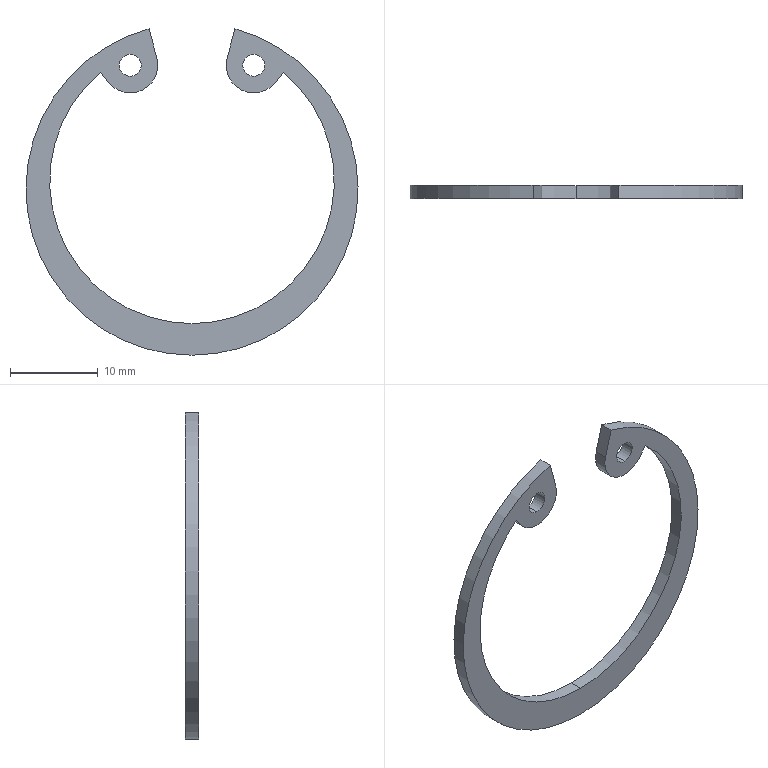Part | SolidWorks | features Extrusion 1 | 1 solid | 18 faces | box 37.8 x 1.5 x 37.156 mm | volume 475.123 mm3 | cylinder 12 | plane 6 | commonest cylinder face diameters 2.5 x4 6.28 x4 32.4 x2 37.8 x2
STEP:
#1=CARTESIAN_POINT('',(7.03,1.5,12.855));
#2=VERTEX_POINT('',#1);
#3=CARTESIAN_POINT('',(7.03,1.5,15.355));
#4=VERTEX_POINT('',#3);
#5=CARTESIAN_POINT('',(7.03,1.5,14.105));
#6=DIRECTION('',(0.,1.,0.));
#7=DIRECTION('',(0.,0.,-1.));
#8=AXIS2_PLACEMENT_3D('',#5,#6,#7);
#9=CIRCLE('',#8,1.25);
#10=EDGE_CURVE('',#2,#4,#9,.T.);
#11=ORIENTED_EDGE('',*,*,#10,.T.);
#12=CARTESIAN_POINT('',(7.03,0.,15.355));
#13=VERTEX_POINT('',#12);
#14=CARTESIAN_POINT('',(7.03,1.5,15.355));
#15=DIRECTION('',(0.,-1.,0.));
#16=VECTOR('',#15,1000.);
#17=LINE('',#14,#16);
#18=EDGE_CURVE('',#4,#13,#17,.T.);
#19=ORIENTED_EDGE('',*,*,#18,.T.);
#20=CARTESIAN_POINT('',(7.03,0.,12.855));
#21=VERTEX_POINT('',#20);
#22=CARTESIAN_POINT('',(7.03,0.,14.105));
#23=DIRECTION('',(0.,1.,0.));
#24=DIRECTION('',(0.,0.,-1.));
#25=AXIS2_PLACEMENT_3D('',#22,#23,#24);
#26=CIRCLE('',#25,1.25);
#27=EDGE_CURVE('',#21,#13,#26,.T.);
#28=ORIENTED_EDGE('',*,*,#27,.F.);
#29=CARTESIAN_POINT('',(7.03,1.5,12.855));
#30=DIRECTION('',(0.,-1.,0.));
#31=VECTOR('',#30,1000.);
#32=LINE('',#29,#31);
#33=EDGE_CURVE('',#2,#21,#32,.T.);
#34=ORIENTED_EDGE('',*,*,#33,.F.);
#35=EDGE_LOOP('',(#11,#19,#28,#34));
#36=FACE_OUTER_BOUND('',#35,.T.);
#37=CARTESIAN_POINT('',(7.03,1.5,14.105));
#38=DIRECTION('',(0.,-1.,0.));
#39=DIRECTION('',(0.,0.,-1.));
#40=AXIS2_PLACEMENT_3D('',#37,#38,#39);
#41=CYLINDRICAL_SURFACE('',#40,1.25);
#42=ADVANCED_FACE('',(#36),#41,.F.);
#43=CARTESIAN_POINT('',(-7.03,1.5,12.855));
#44=VERTEX_POINT('',#43);
#45=CARTESIAN_POINT('',(-7.03,1.5,15.355));
#46=VERTEX_POINT('',#45);
#47=CARTESIAN_POINT('',(-7.03,1.5,14.105));
#48=DIRECTION('',(0.,1.,0.));
#49=DIRECTION('',(0.,0.,1.));
#50=AXIS2_PLACEMENT_3D('',#47,#48,#49);
#51=CIRCLE('',#50,1.25);
#52=EDGE_CURVE('',#44,#46,#51,.T.);
#53=ORIENTED_EDGE('',*,*,#52,.T.);
#54=CARTESIAN_POINT('',(-7.03,0.,15.355));
#55=VERTEX_POINT('',#54);
#56=CARTESIAN_POINT('',(-7.03,1.5,15.355));
#57=DIRECTION('',(0.,-1.,0.));
#58=VECTOR('',#57,1000.);
#59=LINE('',#56,#58);
#60=EDGE_CURVE('',#46,#55,#59,.T.);
#61=ORIENTED_EDGE('',*,*,#60,.T.);
#62=CARTESIAN_POINT('',(-7.03,0.,12.855));
#63=VERTEX_POINT('',#62);
#64=CARTESIAN_POINT('',(-7.03,0.,14.105));
#65=DIRECTION('',(0.,1.,0.));
#66=DIRECTION('',(0.,0.,1.));
#67=AXIS2_PLACEMENT_3D('',#64,#65,#66);
#68=CIRCLE('',#67,1.25);
#69=EDGE_CURVE('',#63,#55,#68,.T.);
#70=ORIENTED_EDGE('',*,*,#69,.F.);
#71=CARTESIAN_POINT('',(-7.03,1.5,12.855));
#72=DIRECTION('',(0.,-1.,0.));
#73=VECTOR('',#72,1000.);
#74=LINE('',#71,#73);
#75=EDGE_CURVE('',#44,#63,#74,.T.);
#76=ORIENTED_EDGE('',*,*,#75,.F.);
#77=EDGE_LOOP('',(#53,#61,#70,#76));
#78=FACE_OUTER_BOUND('',#77,.T.);
#79=CARTESIAN_POINT('',(-7.03,1.5,14.105));
#80=DIRECTION('',(0.,-1.,0.));
#81=DIRECTION('',(0.,0.,-1.));
#82=AXIS2_PLACEMENT_3D('',#79,#80,#81);
#83=CYLINDRICAL_SURFACE('',#82,1.25);
#84=ADVANCED_FACE('',(#78),#83,.F.);
#85=CARTESIAN_POINT('',(0.,1.5,-18.9));
#86=VERTEX_POINT('',#85);
#87=CARTESIAN_POINT('',(-4.892,1.5,18.256));
#88=VERTEX_POINT('',#87);
#89=CARTESIAN_POINT('',(0.,1.5,0.));
#90=DIRECTION('',(0.,1.,0.));
#91=DIRECTION('',(0.,0.,1.));
#92=AXIS2_PLACEMENT_3D('',#89,#90,#91);
#93=CIRCLE('',#92,18.9);
#94=EDGE_CURVE('',#86,#88,#93,.T.);
#95=ORIENTED_EDGE('',*,*,#94,.F.);
#96=CARTESIAN_POINT('',(0.,0.,-18.9));
#97=VERTEX_POINT('',#96);
#98=CARTESIAN_POINT('',(0.,1.5,-18.9));
#99=DIRECTION('',(0.,-1.,0.));
#100=VECTOR('',#99,1000.);
#101=LINE('',#98,#100);
#102=EDGE_CURVE('',#86,#97,#101,.T.);
#103=ORIENTED_EDGE('',*,*,#102,.T.);
#104=CARTESIAN_POINT('',(-4.892,0.,18.256));
#105=VERTEX_POINT('',#104);
#106=CARTESIAN_POINT('',(0.,0.,0.));
#107=DIRECTION('',(0.,1.,0.));
#108=DIRECTION('',(0.,0.,1.));
#109=AXIS2_PLACEMENT_3D('',#106,#107,#108);
#110=CIRCLE('',#109,18.9);
#111=EDGE_CURVE('',#97,#105,#110,.T.);
#112=ORIENTED_EDGE('',*,*,#111,.T.);
#113=CARTESIAN_POINT('',(-4.892,1.5,18.256));
#114=DIRECTION('',(0.,-1.,0.));
#115=VECTOR('',#114,1000.);
#116=LINE('',#113,#115);
#117=EDGE_CURVE('',#88,#105,#116,.T.);
#118=ORIENTED_EDGE('',*,*,#117,.F.);
#119=EDGE_LOOP('',(#95,#103,#112,#118));
#120=FACE_OUTER_BOUND('',#119,.T.);
#121=CARTESIAN_POINT('',(0.,1.5,0.));
#122=DIRECTION('',(0.,-1.,0.));
#123=DIRECTION('',(0.,0.,-1.));
#124=AXIS2_PLACEMENT_3D('',#121,#122,#123);
#125=CYLINDRICAL_SURFACE('',#124,18.9);
#126=ADVANCED_FACE('',(#120),#125,.T.);
#127=CARTESIAN_POINT('',(7.03,1.5,10.965));
#128=VERTEX_POINT('',#127);
#129=CARTESIAN_POINT('',(3.997,1.5,14.918));
#130=VERTEX_POINT('',#129);
#131=CARTESIAN_POINT('',(7.03,1.5,14.105));
#132=DIRECTION('',(0.,1.,0.));
#133=DIRECTION('',(0.,0.,-1.));
#134=AXIS2_PLACEMENT_3D('',#131,#132,#133);
#135=CIRCLE('',#134,3.14);
#136=EDGE_CURVE('',#128,#130,#135,.T.);
#137=ORIENTED_EDGE('',*,*,#136,.F.);
#138=CARTESIAN_POINT('',(7.03,0.,10.965));
#139=VERTEX_POINT('',#138);
#140=CARTESIAN_POINT('',(7.03,1.5,10.965));
#141=DIRECTION('',(0.,-1.,0.));
#142=VECTOR('',#141,1000.);
#143=LINE('',#140,#142);
#144=EDGE_CURVE('',#128,#139,#143,.T.);
#145=ORIENTED_EDGE('',*,*,#144,.T.);
#146=CARTESIAN_POINT('',(3.997,0.,14.918));
#147=VERTEX_POINT('',#146);
#148=CARTESIAN_POINT('',(7.03,0.,14.105));
#149=DIRECTION('',(0.,1.,0.));
#150=DIRECTION('',(0.,0.,-1.));
#151=AXIS2_PLACEMENT_3D('',#148,#149,#150);
#152=CIRCLE('',#151,3.14);
#153=EDGE_CURVE('',#139,#147,#152,.T.);
#154=ORIENTED_EDGE('',*,*,#153,.T.);
#155=CARTESIAN_POINT('',(3.997,1.5,14.918));
#156=DIRECTION('',(0.,-1.,0.));
#157=VECTOR('',#156,1000.);
#158=LINE('',#155,#157);
#159=EDGE_CURVE('',#130,#147,#158,.T.);
#160=ORIENTED_EDGE('',*,*,#159,.F.);
#161=EDGE_LOOP('',(#137,#145,#154,#160));
#162=FACE_OUTER_BOUND('',#161,.T.);
#163=CARTESIAN_POINT('',(7.03,1.5,14.105));
#164=DIRECTION('',(0.,-1.,0.));
#165=DIRECTION('',(0.,0.,-1.));
#166=AXIS2_PLACEMENT_3D('',#163,#164,#165);
#167=CYLINDRICAL_SURFACE('',#166,3.14);
#168=ADVANCED_FACE('',(#162),#167,.T.);
#169=CARTESIAN_POINT('',(0.,1.5,-15.3));
#170=VERTEX_POINT('',#169);
#171=CARTESIAN_POINT('',(10.401,1.5,13.32));
#172=VERTEX_POINT('',#171);
#173=CARTESIAN_POINT('',(0.,1.5,0.9));
#174=DIRECTION('',(0.,-1.,0.));
#175=DIRECTION('',(0.,0.,1.));
#176=AXIS2_PLACEMENT_3D('',#173,#174,#175);
#177=CIRCLE('',#176,16.2);
#178=EDGE_CURVE('',#170,#172,#177,.T.);
#179=ORIENTED_EDGE('',*,*,#178,.F.);
#180=CARTESIAN_POINT('',(0.,0.,-15.3));
#181=VERTEX_POINT('',#180);
#182=CARTESIAN_POINT('',(0.,1.5,-15.3));
#183=DIRECTION('',(0.,-1.,0.));
#184=VECTOR('',#183,1000.);
#185=LINE('',#182,#184);
#186=EDGE_CURVE('',#170,#181,#185,.T.);
#187=ORIENTED_EDGE('',*,*,#186,.T.);
#188=CARTESIAN_POINT('',(10.401,0.,13.32));
#189=VERTEX_POINT('',#188);
#190=CARTESIAN_POINT('',(0.,0.,0.9));
#191=DIRECTION('',(0.,-1.,0.));
#192=DIRECTION('',(0.,0.,1.));
#193=AXIS2_PLACEMENT_3D('',#190,#191,#192);
#194=CIRCLE('',#193,16.2);
#195=EDGE_CURVE('',#181,#189,#194,.T.);
#196=ORIENTED_EDGE('',*,*,#195,.T.);
#197=CARTESIAN_POINT('',(10.401,1.5,13.32));
#198=DIRECTION('',(0.,-1.,0.));
#199=VECTOR('',#198,1000.);
#200=LINE('',#197,#199);
#201=EDGE_CURVE('',#172,#189,#200,.T.);
#202=ORIENTED_EDGE('',*,*,#201,.F.);
#203=EDGE_LOOP('',(#179,#187,#196,#202));
#204=FACE_OUTER_BOUND('',#203,.T.);
#205=CARTESIAN_POINT('',(0.,1.5,0.9));
#206=DIRECTION('',(0.,-1.,0.));
#207=DIRECTION('',(0.,0.,-1.));
#208=AXIS2_PLACEMENT_3D('',#205,#206,#207);
#209=CYLINDRICAL_SURFACE('',#208,16.2);
#210=ADVANCED_FACE('',(#204),#209,.F.);
#211=CARTESIAN_POINT('',(-7.03,1.5,10.965));
#212=VERTEX_POINT('',#211);
#213=CARTESIAN_POINT('',(-9.505,1.5,12.173));
#214=VERTEX_POINT('',#213);
#215=CARTESIAN_POINT('',(-7.03,1.5,14.105));
#216=DIRECTION('',(0.,1.,0.));
#217=DIRECTION('',(0.,0.,1.));
#218=AXIS2_PLACEMENT_3D('',#215,#216,#217);
#219=CIRCLE('',#218,3.14);
#220=EDGE_CURVE('',#212,#214,#219,.T.);
#221=ORIENTED_EDGE('',*,*,#220,.F.);
#222=CARTESIAN_POINT('',(-7.03,0.,10.965));
#223=VERTEX_POINT('',#222);
#224=CARTESIAN_POINT('',(-7.03,1.5,10.965));
#225=DIRECTION('',(0.,-1.,0.));
#226=VECTOR('',#225,1000.);
#227=LINE('',#224,#226);
#228=EDGE_CURVE('',#212,#223,#227,.T.);
#229=ORIENTED_EDGE('',*,*,#228,.T.);
#230=CARTESIAN_POINT('',(-9.505,0.,12.173));
#231=VERTEX_POINT('',#230);
#232=CARTESIAN_POINT('',(-7.03,0.,14.105));
#233=DIRECTION('',(0.,1.,0.));
#234=DIRECTION('',(0.,0.,1.));
#235=AXIS2_PLACEMENT_3D('',#232,#233,#234);
#236=CIRCLE('',#235,3.14);
#237=EDGE_CURVE('',#223,#231,#236,.T.);
#238=ORIENTED_EDGE('',*,*,#237,.T.);
#239=CARTESIAN_POINT('',(-9.505,1.5,12.173));
#240=DIRECTION('',(0.,-1.,0.));
#241=VECTOR('',#240,1000.);
#242=LINE('',#239,#241);
#243=EDGE_CURVE('',#214,#231,#242,.T.);
#244=ORIENTED_EDGE('',*,*,#243,.F.);
#245=EDGE_LOOP('',(#221,#229,#238,#244));
#246=FACE_OUTER_BOUND('',#245,.T.);
#247=CARTESIAN_POINT('',(-7.03,1.5,14.105));
#248=DIRECTION('',(0.,-1.,0.));
#249=DIRECTION('',(0.,0.,-1.));
#250=AXIS2_PLACEMENT_3D('',#247,#248,#249);
#251=CYLINDRICAL_SURFACE('',#250,3.14);
#252=ADVANCED_FACE('',(#246),#251,.T.);
#253=ORIENTED_EDGE('',*,*,#52,.F.);
#254=CARTESIAN_POINT('',(-7.03,1.5,14.105));
#255=DIRECTION('',(0.,1.,0.));
#256=DIRECTION('',(0.,0.,1.));
#257=AXIS2_PLACEMENT_3D('',#254,#255,#256);
#258=CIRCLE('',#257,1.25);
#259=EDGE_CURVE('',#46,#44,#258,.T.);
#260=ORIENTED_EDGE('',*,*,#259,.F.);
#261=EDGE_LOOP('',(#253,#260));
#262=FACE_BOUND('',#261,.T.);
#263=CARTESIAN_POINT('',(-3.997,1.5,14.918));
#264=VERTEX_POINT('',#263);
#265=CARTESIAN_POINT('',(-7.03,1.5,14.105));
#266=DIRECTION('',(0.,1.,0.));
#267=DIRECTION('',(0.,0.,1.));
#268=AXIS2_PLACEMENT_3D('',#265,#266,#267);
#269=CIRCLE('',#268,3.14);
#270=EDGE_CURVE('',#264,#212,#269,.T.);
#271=ORIENTED_EDGE('',*,*,#270,.T.);
#272=ORIENTED_EDGE('',*,*,#220,.T.);
#273=CARTESIAN_POINT('',(-10.401,1.5,13.32));
#274=VERTEX_POINT('',#273);
#275=CARTESIAN_POINT('',(-10.401,1.5,13.32));
#276=DIRECTION('',(-0.6155,0.,0.7882));
#277=VECTOR('',#276,1000.);
#278=LINE('',#275,#277);
#279=EDGE_CURVE('',#214,#274,#278,.T.);
#280=ORIENTED_EDGE('',*,*,#279,.T.);
#281=CARTESIAN_POINT('',(0.,1.5,0.9));
#282=DIRECTION('',(0.,-1.,0.));
#283=DIRECTION('',(0.,0.,1.));
#284=AXIS2_PLACEMENT_3D('',#281,#282,#283);
#285=CIRCLE('',#284,16.2);
#286=EDGE_CURVE('',#274,#170,#285,.T.);
#287=ORIENTED_EDGE('',*,*,#286,.T.);
#288=ORIENTED_EDGE('',*,*,#178,.T.);
#289=CARTESIAN_POINT('',(9.505,1.5,12.173));
#290=VERTEX_POINT('',#289);
#291=CARTESIAN_POINT('',(10.401,1.5,13.32));
#292=DIRECTION('',(-0.6155,0.,-0.7882));
#293=VECTOR('',#292,1000.);
#294=LINE('',#291,#293);
#295=EDGE_CURVE('',#172,#290,#294,.T.);
#296=ORIENTED_EDGE('',*,*,#295,.T.);
#297=CARTESIAN_POINT('',(7.03,1.5,14.105));
#298=DIRECTION('',(0.,1.,0.));
#299=DIRECTION('',(0.,0.,-1.));
#300=AXIS2_PLACEMENT_3D('',#297,#298,#299);
#301=CIRCLE('',#300,3.14);
#302=EDGE_CURVE('',#290,#128,#301,.T.);
#303=ORIENTED_EDGE('',*,*,#302,.T.);
#304=ORIENTED_EDGE('',*,*,#136,.T.);
#305=CARTESIAN_POINT('',(4.892,1.5,18.256));
#306=VERTEX_POINT('',#305);
#307=CARTESIAN_POINT('',(3.997,1.5,14.918));
#308=DIRECTION('',(0.2588,0.,0.9659));
#309=VECTOR('',#308,1000.);
#310=LINE('',#307,#309);
#311=EDGE_CURVE('',#130,#306,#310,.T.);
#312=ORIENTED_EDGE('',*,*,#311,.T.);
#313=CARTESIAN_POINT('',(0.,1.5,0.));
#314=DIRECTION('',(0.,1.,0.));
#315=DIRECTION('',(0.,0.,1.));
#316=AXIS2_PLACEMENT_3D('',#313,#314,#315);
#317=CIRCLE('',#316,18.9);
#318=EDGE_CURVE('',#306,#86,#317,.T.);
#319=ORIENTED_EDGE('',*,*,#318,.T.);
#320=ORIENTED_EDGE('',*,*,#94,.T.);
#321=CARTESIAN_POINT('',(-3.997,1.5,14.918));
#322=DIRECTION('',(0.2588,0.,-0.9659));
#323=VECTOR('',#322,1000.);
#324=LINE('',#321,#323);
#325=EDGE_CURVE('',#88,#264,#324,.T.);
#326=ORIENTED_EDGE('',*,*,#325,.T.);
#327=EDGE_LOOP('',(#271,#272,#280,#287,#288,#296,#303,#304,#312,#319,#320,#326));
#328=FACE_OUTER_BOUND('',#327,.T.);
#329=ORIENTED_EDGE('',*,*,#10,.F.);
#330=CARTESIAN_POINT('',(7.03,1.5,14.105));
#331=DIRECTION('',(0.,1.,0.));
#332=DIRECTION('',(0.,0.,-1.));
#333=AXIS2_PLACEMENT_3D('',#330,#331,#332);
#334=CIRCLE('',#333,1.25);
#335=EDGE_CURVE('',#4,#2,#334,.T.);
#336=ORIENTED_EDGE('',*,*,#335,.F.);
#337=EDGE_LOOP('',(#329,#336));
#338=FACE_BOUND('',#337,.T.);
#339=CARTESIAN_POINT('',(-7.03,1.5,14.105));
#340=DIRECTION('',(0.,1.,0.));
#341=DIRECTION('',(0.,0.,1.));
#342=AXIS2_PLACEMENT_3D('',#339,#340,#341);
#343=PLANE('',#342);
#344=ADVANCED_FACE('',(#262,#328,#338),#343,.T.);
#345=CARTESIAN_POINT('',(-3.997,0.,14.918));
#346=VERTEX_POINT('',#345);
#347=CARTESIAN_POINT('',(-7.03,0.,14.105));
#348=DIRECTION('',(0.,1.,0.));
#349=DIRECTION('',(0.,0.,1.));
#350=AXIS2_PLACEMENT_3D('',#347,#348,#349);
#351=CIRCLE('',#350,3.14);
#352=EDGE_CURVE('',#346,#223,#351,.T.);
#353=ORIENTED_EDGE('',*,*,#352,.F.);
#354=CARTESIAN_POINT('',(-3.997,0.,14.918));
#355=DIRECTION('',(0.2588,0.,-0.9659));
#356=VECTOR('',#355,1000.);
#357=LINE('',#354,#356);
#358=EDGE_CURVE('',#105,#346,#357,.T.);
#359=ORIENTED_EDGE('',*,*,#358,.F.);
#360=ORIENTED_EDGE('',*,*,#111,.F.);
#361=CARTESIAN_POINT('',(4.892,0.,18.256));
#362=VERTEX_POINT('',#361);
#363=CARTESIAN_POINT('',(0.,0.,0.));
#364=DIRECTION('',(0.,1.,0.));
#365=DIRECTION('',(0.,0.,1.));
#366=AXIS2_PLACEMENT_3D('',#363,#364,#365);
#367=CIRCLE('',#366,18.9);
#368=EDGE_CURVE('',#362,#97,#367,.T.);
#369=ORIENTED_EDGE('',*,*,#368,.F.);
#370=CARTESIAN_POINT('',(3.997,0.,14.918));
#371=DIRECTION('',(0.2588,0.,0.9659));
#372=VECTOR('',#371,1000.);
#373=LINE('',#370,#372);
#374=EDGE_CURVE('',#147,#362,#373,.T.);
#375=ORIENTED_EDGE('',*,*,#374,.F.);
#376=ORIENTED_EDGE('',*,*,#153,.F.);
#377=CARTESIAN_POINT('',(9.505,0.,12.173));
#378=VERTEX_POINT('',#377);
#379=CARTESIAN_POINT('',(7.03,0.,14.105));
#380=DIRECTION('',(0.,1.,0.));
#381=DIRECTION('',(0.,0.,-1.));
#382=AXIS2_PLACEMENT_3D('',#379,#380,#381);
#383=CIRCLE('',#382,3.14);
#384=EDGE_CURVE('',#378,#139,#383,.T.);
#385=ORIENTED_EDGE('',*,*,#384,.F.);
#386=CARTESIAN_POINT('',(10.401,0.,13.32));
#387=DIRECTION('',(-0.6155,0.,-0.7882));
#388=VECTOR('',#387,1000.);
#389=LINE('',#386,#388);
#390=EDGE_CURVE('',#189,#378,#389,.T.);
#391=ORIENTED_EDGE('',*,*,#390,.F.);
#392=ORIENTED_EDGE('',*,*,#195,.F.);
#393=CARTESIAN_POINT('',(-10.401,0.,13.32));
#394=VERTEX_POINT('',#393);
#395=CARTESIAN_POINT('',(0.,0.,0.9));
#396=DIRECTION('',(0.,-1.,0.));
#397=DIRECTION('',(0.,0.,1.));
#398=AXIS2_PLACEMENT_3D('',#395,#396,#397);
#399=CIRCLE('',#398,16.2);
#400=EDGE_CURVE('',#394,#181,#399,.T.);
#401=ORIENTED_EDGE('',*,*,#400,.F.);
#402=CARTESIAN_POINT('',(-10.401,0.,13.32));
#403=DIRECTION('',(-0.6155,0.,0.7882));
#404=VECTOR('',#403,1000.);
#405=LINE('',#402,#404);
#406=EDGE_CURVE('',#231,#394,#405,.T.);
#407=ORIENTED_EDGE('',*,*,#406,.F.);
#408=ORIENTED_EDGE('',*,*,#237,.F.);
#409=EDGE_LOOP('',(#353,#359,#360,#369,#375,#376,#385,#391,#392,#401,#407,#408));
#410=FACE_OUTER_BOUND('',#409,.T.);
#411=ORIENTED_EDGE('',*,*,#69,.T.);
#412=CARTESIAN_POINT('',(-7.03,0.,14.105));
#413=DIRECTION('',(0.,1.,0.));
#414=DIRECTION('',(0.,0.,1.));
#415=AXIS2_PLACEMENT_3D('',#412,#413,#414);
#416=CIRCLE('',#415,1.25);
#417=EDGE_CURVE('',#55,#63,#416,.T.);
#418=ORIENTED_EDGE('',*,*,#417,.T.);
#419=EDGE_LOOP('',(#411,#418));
#420=FACE_BOUND('',#419,.T.);
#421=ORIENTED_EDGE('',*,*,#27,.T.);
#422=CARTESIAN_POINT('',(7.03,0.,14.105));
#423=DIRECTION('',(0.,1.,0.));
#424=DIRECTION('',(0.,0.,-1.));
#425=AXIS2_PLACEMENT_3D('',#422,#423,#424);
#426=CIRCLE('',#425,1.25);
#427=EDGE_CURVE('',#13,#21,#426,.T.);
#428=ORIENTED_EDGE('',*,*,#427,.T.);
#429=EDGE_LOOP('',(#421,#428));
#430=FACE_BOUND('',#429,.T.);
#431=CARTESIAN_POINT('',(-7.03,0.,14.105));
#432=DIRECTION('',(0.,1.,0.));
#433=DIRECTION('',(0.,0.,1.));
#434=AXIS2_PLACEMENT_3D('',#431,#432,#433);
#435=PLANE('',#434);
#436=ADVANCED_FACE('',(#410,#420,#430),#435,.F.);
#437=ORIENTED_EDGE('',*,*,#228,.F.);
#438=ORIENTED_EDGE('',*,*,#270,.F.);
#439=CARTESIAN_POINT('',(-3.997,1.5,14.918));
#440=DIRECTION('',(0.,-1.,0.));
#441=VECTOR('',#440,1000.);
#442=LINE('',#439,#441);
#443=EDGE_CURVE('',#264,#346,#442,.T.);
#444=ORIENTED_EDGE('',*,*,#443,.T.);
#445=ORIENTED_EDGE('',*,*,#352,.T.);
#446=EDGE_LOOP('',(#437,#438,#444,#445));
#447=FACE_OUTER_BOUND('',#446,.T.);
#448=CARTESIAN_POINT('',(-7.03,1.5,14.105));
#449=DIRECTION('',(0.,-1.,0.));
#450=DIRECTION('',(0.,0.,-1.));
#451=AXIS2_PLACEMENT_3D('',#448,#449,#450);
#452=CYLINDRICAL_SURFACE('',#451,3.14);
#453=ADVANCED_FACE('',(#447),#452,.T.);
#454=ORIENTED_EDGE('',*,*,#406,.T.);
#455=CARTESIAN_POINT('',(-10.401,1.5,13.32));
#456=DIRECTION('',(0.,-1.,0.));
#457=VECTOR('',#456,1000.);
#458=LINE('',#455,#457);
#459=EDGE_CURVE('',#274,#394,#458,.T.);
#460=ORIENTED_EDGE('',*,*,#459,.F.);
#461=ORIENTED_EDGE('',*,*,#279,.F.);
#462=ORIENTED_EDGE('',*,*,#243,.T.);
#463=EDGE_LOOP('',(#454,#460,#461,#462));
#464=FACE_OUTER_BOUND('',#463,.T.);
#465=CARTESIAN_POINT('',(-10.401,1.5,13.32));
#466=DIRECTION('',(0.7882,0.,0.6155));
#467=DIRECTION('',(0.6155,0.,-0.7882));
#468=AXIS2_PLACEMENT_3D('',#465,#466,#467);
#469=PLANE('',#468);
#470=ADVANCED_FACE('',(#464),#469,.F.);
#471=ORIENTED_EDGE('',*,*,#186,.F.);
#472=ORIENTED_EDGE('',*,*,#286,.F.);
#473=ORIENTED_EDGE('',*,*,#459,.T.);
#474=ORIENTED_EDGE('',*,*,#400,.T.);
#475=EDGE_LOOP('',(#471,#472,#473,#474));
#476=FACE_OUTER_BOUND('',#475,.T.);
#477=CARTESIAN_POINT('',(0.,1.5,0.9));
#478=DIRECTION('',(0.,-1.,0.));
#479=DIRECTION('',(0.,0.,-1.));
#480=AXIS2_PLACEMENT_3D('',#477,#478,#479);
#481=CYLINDRICAL_SURFACE('',#480,16.2);
#482=ADVANCED_FACE('',(#476),#481,.F.);
#483=ORIENTED_EDGE('',*,*,#390,.T.);
#484=CARTESIAN_POINT('',(9.505,1.5,12.173));
#485=DIRECTION('',(0.,-1.,0.));
#486=VECTOR('',#485,1000.);
#487=LINE('',#484,#486);
#488=EDGE_CURVE('',#290,#378,#487,.T.);
#489=ORIENTED_EDGE('',*,*,#488,.F.);
#490=ORIENTED_EDGE('',*,*,#295,.F.);
#491=ORIENTED_EDGE('',*,*,#201,.T.);
#492=EDGE_LOOP('',(#483,#489,#490,#491));
#493=FACE_OUTER_BOUND('',#492,.T.);
#494=CARTESIAN_POINT('',(10.401,1.5,13.32));
#495=DIRECTION('',(-0.7882,0.,0.6155));
#496=DIRECTION('',(0.6155,0.,0.7882));
#497=AXIS2_PLACEMENT_3D('',#494,#495,#496);
#498=PLANE('',#497);
#499=ADVANCED_FACE('',(#493),#498,.F.);
#500=ORIENTED_EDGE('',*,*,#144,.F.);
#501=ORIENTED_EDGE('',*,*,#302,.F.);
#502=ORIENTED_EDGE('',*,*,#488,.T.);
#503=ORIENTED_EDGE('',*,*,#384,.T.);
#504=EDGE_LOOP('',(#500,#501,#502,#503));
#505=FACE_OUTER_BOUND('',#504,.T.);
#506=CARTESIAN_POINT('',(7.03,1.5,14.105));
#507=DIRECTION('',(0.,-1.,0.));
#508=DIRECTION('',(0.,0.,-1.));
#509=AXIS2_PLACEMENT_3D('',#506,#507,#508);
#510=CYLINDRICAL_SURFACE('',#509,3.14);
#511=ADVANCED_FACE('',(#505),#510,.T.);
#512=ORIENTED_EDGE('',*,*,#374,.T.);
#513=CARTESIAN_POINT('',(4.892,1.5,18.256));
#514=DIRECTION('',(0.,-1.,0.));
#515=VECTOR('',#514,1000.);
#516=LINE('',#513,#515);
#517=EDGE_CURVE('',#306,#362,#516,.T.);
#518=ORIENTED_EDGE('',*,*,#517,.F.);
#519=ORIENTED_EDGE('',*,*,#311,.F.);
#520=ORIENTED_EDGE('',*,*,#159,.T.);
#521=EDGE_LOOP('',(#512,#518,#519,#520));
#522=FACE_OUTER_BOUND('',#521,.T.);
#523=CARTESIAN_POINT('',(3.997,1.5,14.918));
#524=DIRECTION('',(0.9659,0.,-0.2588));
#525=DIRECTION('',(-0.2588,0.,-0.9659));
#526=AXIS2_PLACEMENT_3D('',#523,#524,#525);
#527=PLANE('',#526);
#528=ADVANCED_FACE('',(#522),#527,.F.);
#529=ORIENTED_EDGE('',*,*,#102,.F.);
#530=ORIENTED_EDGE('',*,*,#318,.F.);
#531=ORIENTED_EDGE('',*,*,#517,.T.);
#532=ORIENTED_EDGE('',*,*,#368,.T.);
#533=EDGE_LOOP('',(#529,#530,#531,#532));
#534=FACE_OUTER_BOUND('',#533,.T.);
#535=CARTESIAN_POINT('',(0.,1.5,0.));
#536=DIRECTION('',(0.,-1.,0.));
#537=DIRECTION('',(0.,0.,-1.));
#538=AXIS2_PLACEMENT_3D('',#535,#536,#537);
#539=CYLINDRICAL_SURFACE('',#538,18.9);
#540=ADVANCED_FACE('',(#534),#539,.T.);
#541=ORIENTED_EDGE('',*,*,#358,.T.);
#542=ORIENTED_EDGE('',*,*,#443,.F.);
#543=ORIENTED_EDGE('',*,*,#325,.F.);
#544=ORIENTED_EDGE('',*,*,#117,.T.);
#545=EDGE_LOOP('',(#541,#542,#543,#544));
#546=FACE_OUTER_BOUND('',#545,.T.);
#547=CARTESIAN_POINT('',(-3.997,1.5,14.918));
#548=DIRECTION('',(-0.9659,0.,-0.2588));
#549=DIRECTION('',(-0.2588,0.,0.9659));
#550=AXIS2_PLACEMENT_3D('',#547,#548,#549);
#551=PLANE('',#550);
#552=ADVANCED_FACE('',(#546),#551,.F.);
#553=ORIENTED_EDGE('',*,*,#60,.F.);
#554=ORIENTED_EDGE('',*,*,#259,.T.);
#555=ORIENTED_EDGE('',*,*,#75,.T.);
#556=ORIENTED_EDGE('',*,*,#417,.F.);
#557=EDGE_LOOP('',(#553,#554,#555,#556));
#558=FACE_OUTER_BOUND('',#557,.T.);
#559=CARTESIAN_POINT('',(-7.03,1.5,14.105));
#560=DIRECTION('',(0.,-1.,0.));
#561=DIRECTION('',(0.,0.,-1.));
#562=AXIS2_PLACEMENT_3D('',#559,#560,#561);
#563=CYLINDRICAL_SURFACE('',#562,1.25);
#564=ADVANCED_FACE('',(#558),#563,.F.);
#565=ORIENTED_EDGE('',*,*,#18,.F.);
#566=ORIENTED_EDGE('',*,*,#335,.T.);
#567=ORIENTED_EDGE('',*,*,#33,.T.);
#568=ORIENTED_EDGE('',*,*,#427,.F.);
#569=EDGE_LOOP('',(#565,#566,#567,#568));
#570=FACE_OUTER_BOUND('',#569,.T.);
#571=CARTESIAN_POINT('',(7.03,1.5,14.105));
#572=DIRECTION('',(0.,-1.,0.));
#573=DIRECTION('',(0.,0.,-1.));
#574=AXIS2_PLACEMENT_3D('',#571,#572,#573);
#575=CYLINDRICAL_SURFACE('',#574,1.25);
#576=ADVANCED_FACE('',(#570),#575,.F.);
#577=CLOSED_SHELL('',(#42,#84,#126,#168,#210,#252,#344,#436,#453,#470,#482,#499,#511,#528,#540,#552,#564,#576));
#578=MANIFOLD_SOLID_BREP('',#577);
#579=CARTESIAN_POINT('',(0.,0.,0.));
#580=DIRECTION('',(0.,0.,1.));
#581=DIRECTION('',(1.,0.,0.));
#582=AXIS2_PLACEMENT_3D('',#579,#580,#581);
#583=(LENGTH_UNIT()NAMED_UNIT(*)SI_UNIT(.MILLI.,.METRE.));
#584=UNCERTAINTY_MEASURE_WITH_UNIT(LENGTH_MEASURE(0.00001),#583,'','');
#585=(NAMED_UNIT(*)PLANE_ANGLE_UNIT()SI_UNIT($,.RADIAN.));
#586=(NAMED_UNIT(*)SI_UNIT($,.STERADIAN.)SOLID_ANGLE_UNIT());
#587=(GEOMETRIC_REPRESENTATION_CONTEXT(3)GLOBAL_UNCERTAINTY_ASSIGNED_CONTEXT((#584))GLOBAL_UNIT_ASSIGNED_CONTEXT((#583,#585,#586))REPRESENTATION_CONTEXT('',''));
#588=ADVANCED_BREP_SHAPE_REPRESENTATION('',(#578,#582),#587);